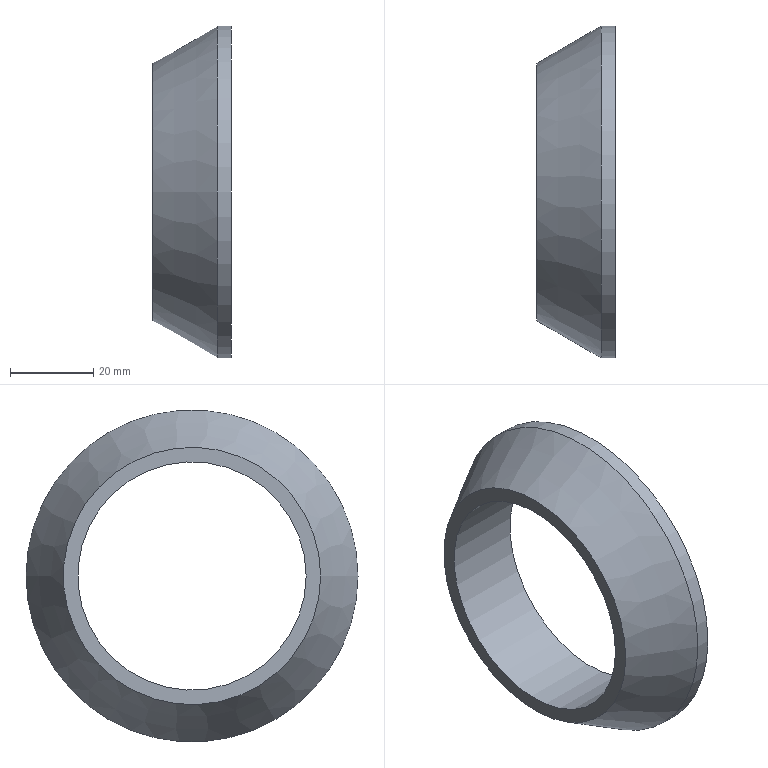Part | NX | features solid 2 | 1 solid | 5 faces | box 19 x 80 x 80 mm | volume 34056 mm3 | cylinder 2 | plane 2 | cone 1 | commonest cylinder face diameters 55 x1 80 x1
STEP:
#1=CARTESIAN_POINT('',(1835.,-1237.5,-487.5));
#2=VERTEX_POINT('',#1);
#3=CARTESIAN_POINT('',(1835.,-1210.,-487.5));
#4=DIRECTION('',(-1.,0.,0.));
#5=DIRECTION('',(0.,-1.,0.));
#6=AXIS2_PLACEMENT_3D('',#3,#4,#5);
#7=CIRCLE('',#6,27.5);
#8=EDGE_CURVE('',#2,#2,#7,.T.);
#9=ORIENTED_EDGE('',*,*,#8,.T.);
#10=EDGE_LOOP('',(#9));
#11=FACE_BOUND('',#10,.T.);
#12=CARTESIAN_POINT('',(1854.,-1237.5,-487.5));
#13=VERTEX_POINT('',#12);
#14=CARTESIAN_POINT('',(1854.,-1210.,-487.5));
#15=DIRECTION('',(-1.,0.,0.));
#16=DIRECTION('',(0.,-1.,0.));
#17=AXIS2_PLACEMENT_3D('',#14,#15,#16);
#18=CIRCLE('',#17,27.5);
#19=EDGE_CURVE('',#13,#13,#18,.T.);
#20=ORIENTED_EDGE('',*,*,#19,.F.);
#21=EDGE_LOOP('',(#20));
#22=FACE_BOUND('',#21,.T.);
#23=CARTESIAN_POINT('',(1835.,-1210.,-487.5));
#24=DIRECTION('',(1.,0.,0.));
#25=DIRECTION('',(0.,-1.,0.));
#26=AXIS2_PLACEMENT_3D('',#23,#24,#25);
#27=CYLINDRICAL_SURFACE('',#26,27.5);
#28=ADVANCED_FACE('',(#11,#22),#27,.F.);
#29=CARTESIAN_POINT('',(1850.588,-1250.,-487.5));
#30=VERTEX_POINT('',#29);
#31=CARTESIAN_POINT('',(1850.588,-1210.,-487.5));
#32=DIRECTION('',(-1.,0.,0.));
#33=DIRECTION('',(0.,-1.,0.));
#34=AXIS2_PLACEMENT_3D('',#31,#32,#33);
#35=CIRCLE('',#34,40.);
#36=EDGE_CURVE('',#30,#30,#35,.T.);
#37=ORIENTED_EDGE('',*,*,#36,.F.);
#38=EDGE_LOOP('',(#37));
#39=FACE_BOUND('',#38,.T.);
#40=CARTESIAN_POINT('',(1854.,-1250.,-487.5));
#41=VERTEX_POINT('',#40);
#42=CARTESIAN_POINT('',(1854.,-1210.,-487.5));
#43=DIRECTION('',(-1.,0.,0.));
#44=DIRECTION('',(0.,-1.,0.));
#45=AXIS2_PLACEMENT_3D('',#42,#43,#44);
#46=CIRCLE('',#45,40.);
#47=EDGE_CURVE('',#41,#41,#46,.T.);
#48=ORIENTED_EDGE('',*,*,#47,.T.);
#49=EDGE_LOOP('',(#48));
#50=FACE_BOUND('',#49,.T.);
#51=CARTESIAN_POINT('',(1835.,-1210.,-487.5));
#52=DIRECTION('',(1.,0.,0.));
#53=DIRECTION('',(0.,-1.,0.));
#54=AXIS2_PLACEMENT_3D('',#51,#52,#53);
#55=CYLINDRICAL_SURFACE('',#54,40.);
#56=ADVANCED_FACE('',(#39,#50),#55,.T.);
#57=CARTESIAN_POINT('',(1835.,-1241.,-487.5));
#58=VERTEX_POINT('',#57);
#59=CARTESIAN_POINT('',(1835.,-1210.,-487.5));
#60=DIRECTION('',(-1.,0.,0.));
#61=DIRECTION('',(0.,-1.,0.));
#62=AXIS2_PLACEMENT_3D('',#59,#60,#61);
#63=CIRCLE('',#62,31.);
#64=EDGE_CURVE('',#58,#58,#63,.F.);
#65=ORIENTED_EDGE('',*,*,#64,.F.);
#66=EDGE_LOOP('',(#65));
#67=FACE_BOUND('',#66,.T.);
#68=ORIENTED_EDGE('',*,*,#8,.F.);
#69=EDGE_LOOP('',(#68));
#70=FACE_BOUND('',#69,.T.);
#71=CARTESIAN_POINT('',(1835.,-1210.,-487.5));
#72=DIRECTION('',(1.,0.,0.));
#73=DIRECTION('',(0.,-1.,0.));
#74=AXIS2_PLACEMENT_3D('',#71,#72,#73);
#75=PLANE('',#74);
#76=ADVANCED_FACE('',(#67,#70),#75,.F.);
#77=ORIENTED_EDGE('',*,*,#19,.T.);
#78=EDGE_LOOP('',(#77));
#79=FACE_BOUND('',#78,.T.);
#80=ORIENTED_EDGE('',*,*,#47,.F.);
#81=EDGE_LOOP('',(#80));
#82=FACE_BOUND('',#81,.T.);
#83=CARTESIAN_POINT('',(1854.,-1210.,-487.5));
#84=DIRECTION('',(1.,0.,0.));
#85=DIRECTION('',(0.,-1.,0.));
#86=AXIS2_PLACEMENT_3D('',#83,#84,#85);
#87=PLANE('',#86);
#88=ADVANCED_FACE('',(#79,#82),#87,.T.);
#89=ORIENTED_EDGE('',*,*,#64,.T.);
#90=EDGE_LOOP('',(#89));
#91=FACE_BOUND('',#90,.T.);
#92=ORIENTED_EDGE('',*,*,#36,.T.);
#93=EDGE_LOOP('',(#92));
#94=FACE_BOUND('',#93,.T.);
#95=CARTESIAN_POINT('',(1850.588,-1210.,-487.5));
#96=DIRECTION('',(1.,0.,0.));
#97=DIRECTION('',(0.,-1.,0.));
#98=AXIS2_PLACEMENT_3D('',#95,#96,#97);
#99=CONICAL_SURFACE('',#98,40.,0.5236);
#100=ADVANCED_FACE('',(#91,#94),#99,.T.);
#101=CLOSED_SHELL('',(#28,#56,#76,#88,#100));
#102=MANIFOLD_SOLID_BREP('',#101);
#103=(LENGTH_UNIT()NAMED_UNIT(*)SI_UNIT(.MILLI.,.METRE.));
#104=UNCERTAINTY_MEASURE_WITH_UNIT(LENGTH_MEASURE(0.00001),#103,'','');
#105=(NAMED_UNIT(*)PLANE_ANGLE_UNIT()SI_UNIT($,.RADIAN.));
#106=(NAMED_UNIT(*)SI_UNIT($,.STERADIAN.)SOLID_ANGLE_UNIT());
#107=(GEOMETRIC_REPRESENTATION_CONTEXT(3)GLOBAL_UNCERTAINTY_ASSIGNED_CONTEXT((#104))GLOBAL_UNIT_ASSIGNED_CONTEXT((#103,#105,#106))REPRESENTATION_CONTEXT('',''));
#108=ADVANCED_BREP_SHAPE_REPRESENTATION('',(#102),#107);